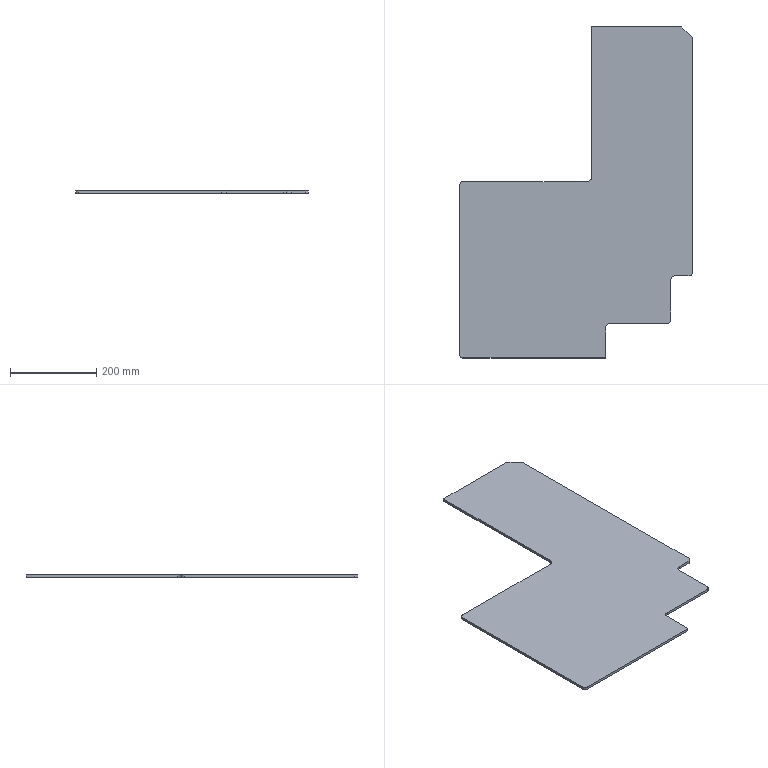Part | SolidWorks | features FlatPattern 1, SMBaseFlange 1, SheetMetal 1 | 1 solid | 24 faces | box 538 x 768 x 6 mm | volume 1689315 mm3 | plane 13 | cylinder 11 | commonest cylinder face diameters 15 x6 21 x3 3 x2
STEP:
#1=CARTESIAN_POINT('',(215.211,367.287,0.));
#2=VERTEX_POINT('',#1);
#3=CARTESIAN_POINT('',(209.908,369.483,0.));
#4=VERTEX_POINT('',#3);
#5=CARTESIAN_POINT('',(209.908,361.983,0.));
#6=DIRECTION('',(0.,0.,1.));
#7=DIRECTION('',(1.,0.,0.));
#8=AXIS2_PLACEMENT_3D('',#5,#6,#7);
#9=CIRCLE('',#8,7.5);
#10=EDGE_CURVE('',#2,#4,#9,.T.);
#11=ORIENTED_EDGE('',*,*,#10,.F.);
#12=CARTESIAN_POINT('',(215.211,367.287,-6.));
#13=VERTEX_POINT('',#12);
#14=CARTESIAN_POINT('',(215.211,367.287,-6.));
#15=DIRECTION('',(0.,0.,1.));
#16=VECTOR('',#15,1000.);
#17=LINE('',#14,#16);
#18=EDGE_CURVE('',#13,#2,#17,.T.);
#19=ORIENTED_EDGE('',*,*,#18,.F.);
#20=CARTESIAN_POINT('',(209.908,369.483,-6.));
#21=VERTEX_POINT('',#20);
#22=CARTESIAN_POINT('',(209.908,361.983,-6.));
#23=DIRECTION('',(0.,0.,1.));
#24=DIRECTION('',(1.,0.,0.));
#25=AXIS2_PLACEMENT_3D('',#22,#23,#24);
#26=CIRCLE('',#25,7.5);
#27=EDGE_CURVE('',#13,#21,#26,.T.);
#28=ORIENTED_EDGE('',*,*,#27,.T.);
#29=CARTESIAN_POINT('',(209.908,369.483,-6.));
#30=DIRECTION('',(0.,0.,1.));
#31=VECTOR('',#30,1000.);
#32=LINE('',#29,#31);
#33=EDGE_CURVE('',#21,#4,#32,.T.);
#34=ORIENTED_EDGE('',*,*,#33,.T.);
#35=EDGE_LOOP('',(#11,#19,#28,#34));
#36=FACE_OUTER_BOUND('',#35,.T.);
#37=CARTESIAN_POINT('',(209.908,361.983,-6.));
#38=DIRECTION('',(0.,0.,1.));
#39=DIRECTION('',(1.,0.,0.));
#40=AXIS2_PLACEMENT_3D('',#37,#38,#39);
#41=CYLINDRICAL_SURFACE('',#40,7.5);
#42=ADVANCED_FACE('',(#36),#41,.T.);
#43=CARTESIAN_POINT('',(237.303,345.195,0.));
#44=VERTEX_POINT('',#43);
#45=CARTESIAN_POINT('',(237.303,345.195,0.));
#46=DIRECTION('',(-0.7071,0.7071,0.));
#47=VECTOR('',#46,1000.);
#48=LINE('',#45,#47);
#49=EDGE_CURVE('',#44,#2,#48,.T.);
#50=ORIENTED_EDGE('',*,*,#49,.F.);
#51=CARTESIAN_POINT('',(237.303,345.195,-6.));
#52=VERTEX_POINT('',#51);
#53=CARTESIAN_POINT('',(237.303,345.195,-6.));
#54=DIRECTION('',(0.,0.,1.));
#55=VECTOR('',#54,1000.);
#56=LINE('',#53,#55);
#57=EDGE_CURVE('',#52,#44,#56,.T.);
#58=ORIENTED_EDGE('',*,*,#57,.F.);
#59=CARTESIAN_POINT('',(237.303,345.195,-6.));
#60=DIRECTION('',(-0.7071,0.7071,0.));
#61=VECTOR('',#60,1000.);
#62=LINE('',#59,#61);
#63=EDGE_CURVE('',#52,#13,#62,.T.);
#64=ORIENTED_EDGE('',*,*,#63,.T.);
#65=ORIENTED_EDGE('',*,*,#18,.T.);
#66=EDGE_LOOP('',(#50,#58,#64,#65));
#67=FACE_OUTER_BOUND('',#66,.T.);
#68=CARTESIAN_POINT('',(237.303,345.195,-6.));
#69=DIRECTION('',(0.7071,0.7071,0.));
#70=DIRECTION('',(-0.7071,0.7071,0.));
#71=AXIS2_PLACEMENT_3D('',#68,#69,#70);
#72=PLANE('',#71);
#73=ADVANCED_FACE('',(#67),#72,.T.);
#74=CARTESIAN_POINT('',(239.5,339.892,0.));
#75=VERTEX_POINT('',#74);
#76=CARTESIAN_POINT('',(232.,339.892,0.));
#77=DIRECTION('',(0.,0.,1.));
#78=DIRECTION('',(1.,0.,0.));
#79=AXIS2_PLACEMENT_3D('',#76,#77,#78);
#80=CIRCLE('',#79,7.5);
#81=EDGE_CURVE('',#75,#44,#80,.T.);
#82=ORIENTED_EDGE('',*,*,#81,.F.);
#83=CARTESIAN_POINT('',(239.5,339.892,-6.));
#84=VERTEX_POINT('',#83);
#85=CARTESIAN_POINT('',(239.5,339.892,-6.));
#86=DIRECTION('',(0.,0.,1.));
#87=VECTOR('',#86,1000.);
#88=LINE('',#85,#87);
#89=EDGE_CURVE('',#84,#75,#88,.T.);
#90=ORIENTED_EDGE('',*,*,#89,.F.);
#91=CARTESIAN_POINT('',(232.,339.892,-6.));
#92=DIRECTION('',(0.,0.,1.));
#93=DIRECTION('',(1.,0.,0.));
#94=AXIS2_PLACEMENT_3D('',#91,#92,#93);
#95=CIRCLE('',#94,7.5);
#96=EDGE_CURVE('',#84,#52,#95,.T.);
#97=ORIENTED_EDGE('',*,*,#96,.T.);
#98=ORIENTED_EDGE('',*,*,#57,.T.);
#99=EDGE_LOOP('',(#82,#90,#97,#98));
#100=FACE_OUTER_BOUND('',#99,.T.);
#101=CARTESIAN_POINT('',(232.,339.892,-6.));
#102=DIRECTION('',(0.,0.,1.));
#103=DIRECTION('',(1.,0.,0.));
#104=AXIS2_PLACEMENT_3D('',#101,#102,#103);
#105=CYLINDRICAL_SURFACE('',#104,7.5);
#106=ADVANCED_FACE('',(#100),#105,.T.);
#107=CARTESIAN_POINT('',(239.5,-201.017,0.));
#108=VERTEX_POINT('',#107);
#109=CARTESIAN_POINT('',(239.5,-201.017,0.));
#110=DIRECTION('',(0.,1.,0.));
#111=VECTOR('',#110,1000.);
#112=LINE('',#109,#111);
#113=EDGE_CURVE('',#108,#75,#112,.T.);
#114=ORIENTED_EDGE('',*,*,#113,.F.);
#115=CARTESIAN_POINT('',(239.5,-201.017,-6.));
#116=VERTEX_POINT('',#115);
#117=CARTESIAN_POINT('',(239.5,-201.017,-6.));
#118=DIRECTION('',(0.,0.,1.));
#119=VECTOR('',#118,1000.);
#120=LINE('',#117,#119);
#121=EDGE_CURVE('',#116,#108,#120,.T.);
#122=ORIENTED_EDGE('',*,*,#121,.F.);
#123=CARTESIAN_POINT('',(239.5,-201.017,-6.));
#124=DIRECTION('',(0.,1.,0.));
#125=VECTOR('',#124,1000.);
#126=LINE('',#123,#125);
#127=EDGE_CURVE('',#116,#84,#126,.T.);
#128=ORIENTED_EDGE('',*,*,#127,.T.);
#129=ORIENTED_EDGE('',*,*,#89,.T.);
#130=EDGE_LOOP('',(#114,#122,#128,#129));
#131=FACE_OUTER_BOUND('',#130,.T.);
#132=CARTESIAN_POINT('',(239.5,-201.017,-6.));
#133=DIRECTION('',(1.,0.,0.));
#134=DIRECTION('',(0.,0.,-1.));
#135=AXIS2_PLACEMENT_3D('',#132,#133,#134);
#136=PLANE('',#135);
#137=ADVANCED_FACE('',(#131),#136,.T.);
#138=CARTESIAN_POINT('',(232.,-208.517,0.));
#139=VERTEX_POINT('',#138);
#140=CARTESIAN_POINT('',(232.,-201.017,0.));
#141=DIRECTION('',(0.,0.,1.));
#142=DIRECTION('',(-1.,0.,0.));
#143=AXIS2_PLACEMENT_3D('',#140,#141,#142);
#144=CIRCLE('',#143,7.5);
#145=EDGE_CURVE('',#139,#108,#144,.T.);
#146=ORIENTED_EDGE('',*,*,#145,.F.);
#147=CARTESIAN_POINT('',(232.,-208.517,-6.));
#148=VERTEX_POINT('',#147);
#149=CARTESIAN_POINT('',(232.,-208.517,-6.));
#150=DIRECTION('',(0.,0.,1.));
#151=VECTOR('',#150,1000.);
#152=LINE('',#149,#151);
#153=EDGE_CURVE('',#148,#139,#152,.T.);
#154=ORIENTED_EDGE('',*,*,#153,.F.);
#155=CARTESIAN_POINT('',(232.,-201.017,-6.));
#156=DIRECTION('',(0.,0.,1.));
#157=DIRECTION('',(-1.,0.,0.));
#158=AXIS2_PLACEMENT_3D('',#155,#156,#157);
#159=CIRCLE('',#158,7.5);
#160=EDGE_CURVE('',#148,#116,#159,.T.);
#161=ORIENTED_EDGE('',*,*,#160,.T.);
#162=ORIENTED_EDGE('',*,*,#121,.T.);
#163=EDGE_LOOP('',(#146,#154,#161,#162));
#164=FACE_OUTER_BOUND('',#163,.T.);
#165=CARTESIAN_POINT('',(232.,-201.017,-6.));
#166=DIRECTION('',(0.,0.,1.));
#167=DIRECTION('',(1.,0.,0.));
#168=AXIS2_PLACEMENT_3D('',#165,#166,#167);
#169=CYLINDRICAL_SURFACE('',#168,7.5);
#170=ADVANCED_FACE('',(#164),#169,.T.);
#171=CARTESIAN_POINT('',(200.,-208.517,0.));
#172=VERTEX_POINT('',#171);
#173=CARTESIAN_POINT('',(200.,-208.517,0.));
#174=DIRECTION('',(1.,0.,0.));
#175=VECTOR('',#174,1000.);
#176=LINE('',#173,#175);
#177=EDGE_CURVE('',#172,#139,#176,.T.);
#178=ORIENTED_EDGE('',*,*,#177,.F.);
#179=CARTESIAN_POINT('',(200.,-208.517,-6.));
#180=VERTEX_POINT('',#179);
#181=CARTESIAN_POINT('',(200.,-208.517,-6.));
#182=DIRECTION('',(0.,0.,1.));
#183=VECTOR('',#182,1000.);
#184=LINE('',#181,#183);
#185=EDGE_CURVE('',#180,#172,#184,.T.);
#186=ORIENTED_EDGE('',*,*,#185,.F.);
#187=CARTESIAN_POINT('',(200.,-208.517,-6.));
#188=DIRECTION('',(1.,0.,0.));
#189=VECTOR('',#188,1000.);
#190=LINE('',#187,#189);
#191=EDGE_CURVE('',#180,#148,#190,.T.);
#192=ORIENTED_EDGE('',*,*,#191,.T.);
#193=ORIENTED_EDGE('',*,*,#153,.T.);
#194=EDGE_LOOP('',(#178,#186,#192,#193));
#195=FACE_OUTER_BOUND('',#194,.T.);
#196=CARTESIAN_POINT('',(200.,-208.517,-6.));
#197=DIRECTION('',(0.,-1.,0.));
#198=DIRECTION('',(0.,0.,-1.));
#199=AXIS2_PLACEMENT_3D('',#196,#197,#198);
#200=PLANE('',#199);
#201=ADVANCED_FACE('',(#195),#200,.T.);
#202=CARTESIAN_POINT('',(189.5,-219.017,0.));
#203=VERTEX_POINT('',#202);
#204=CARTESIAN_POINT('',(200.,-219.017,0.));
#205=DIRECTION('',(0.,0.,-1.));
#206=DIRECTION('',(1.,0.,0.));
#207=AXIS2_PLACEMENT_3D('',#204,#205,#206);
#208=CIRCLE('',#207,10.5);
#209=EDGE_CURVE('',#203,#172,#208,.T.);
#210=ORIENTED_EDGE('',*,*,#209,.F.);
#211=CARTESIAN_POINT('',(189.5,-219.017,-6.));
#212=VERTEX_POINT('',#211);
#213=CARTESIAN_POINT('',(189.5,-219.017,-6.));
#214=DIRECTION('',(0.,0.,1.));
#215=VECTOR('',#214,1000.);
#216=LINE('',#213,#215);
#217=EDGE_CURVE('',#212,#203,#216,.T.);
#218=ORIENTED_EDGE('',*,*,#217,.F.);
#219=CARTESIAN_POINT('',(200.,-219.017,-6.));
#220=DIRECTION('',(0.,0.,-1.));
#221=DIRECTION('',(1.,0.,0.));
#222=AXIS2_PLACEMENT_3D('',#219,#220,#221);
#223=CIRCLE('',#222,10.5);
#224=EDGE_CURVE('',#212,#180,#223,.T.);
#225=ORIENTED_EDGE('',*,*,#224,.T.);
#226=ORIENTED_EDGE('',*,*,#185,.T.);
#227=EDGE_LOOP('',(#210,#218,#225,#226));
#228=FACE_OUTER_BOUND('',#227,.T.);
#229=CARTESIAN_POINT('',(200.,-219.017,-6.));
#230=DIRECTION('',(0.,0.,1.));
#231=DIRECTION('',(1.,0.,0.));
#232=AXIS2_PLACEMENT_3D('',#229,#230,#231);
#233=CYLINDRICAL_SURFACE('',#232,10.5);
#234=ADVANCED_FACE('',(#228),#233,.F.);
#235=CARTESIAN_POINT('',(189.5,-311.017,0.));
#236=VERTEX_POINT('',#235);
#237=CARTESIAN_POINT('',(189.5,-311.017,0.));
#238=DIRECTION('',(0.,1.,0.));
#239=VECTOR('',#238,1000.);
#240=LINE('',#237,#239);
#241=EDGE_CURVE('',#236,#203,#240,.T.);
#242=ORIENTED_EDGE('',*,*,#241,.F.);
#243=CARTESIAN_POINT('',(189.5,-311.017,-6.));
#244=VERTEX_POINT('',#243);
#245=CARTESIAN_POINT('',(189.5,-311.017,-6.));
#246=DIRECTION('',(0.,0.,1.));
#247=VECTOR('',#246,1000.);
#248=LINE('',#245,#247);
#249=EDGE_CURVE('',#244,#236,#248,.T.);
#250=ORIENTED_EDGE('',*,*,#249,.F.);
#251=CARTESIAN_POINT('',(189.5,-311.017,-6.));
#252=DIRECTION('',(0.,1.,0.));
#253=VECTOR('',#252,1000.);
#254=LINE('',#251,#253);
#255=EDGE_CURVE('',#244,#212,#254,.T.);
#256=ORIENTED_EDGE('',*,*,#255,.T.);
#257=ORIENTED_EDGE('',*,*,#217,.T.);
#258=EDGE_LOOP('',(#242,#250,#256,#257));
#259=FACE_OUTER_BOUND('',#258,.T.);
#260=CARTESIAN_POINT('',(189.5,-311.017,-6.));
#261=DIRECTION('',(1.,0.,0.));
#262=DIRECTION('',(0.,0.,-1.));
#263=AXIS2_PLACEMENT_3D('',#260,#261,#262);
#264=PLANE('',#263);
#265=ADVANCED_FACE('',(#259),#264,.T.);
#266=CARTESIAN_POINT('',(182.,-318.517,0.));
#267=VERTEX_POINT('',#266);
#268=CARTESIAN_POINT('',(182.,-311.017,0.));
#269=DIRECTION('',(0.,0.,1.));
#270=DIRECTION('',(-1.,0.,0.));
#271=AXIS2_PLACEMENT_3D('',#268,#269,#270);
#272=CIRCLE('',#271,7.5);
#273=EDGE_CURVE('',#267,#236,#272,.T.);
#274=ORIENTED_EDGE('',*,*,#273,.F.);
#275=CARTESIAN_POINT('',(182.,-318.517,-6.));
#276=VERTEX_POINT('',#275);
#277=CARTESIAN_POINT('',(182.,-318.517,-6.));
#278=DIRECTION('',(0.,0.,1.));
#279=VECTOR('',#278,1000.);
#280=LINE('',#277,#279);
#281=EDGE_CURVE('',#276,#267,#280,.T.);
#282=ORIENTED_EDGE('',*,*,#281,.F.);
#283=CARTESIAN_POINT('',(182.,-311.017,-6.));
#284=DIRECTION('',(0.,0.,1.));
#285=DIRECTION('',(-1.,0.,0.));
#286=AXIS2_PLACEMENT_3D('',#283,#284,#285);
#287=CIRCLE('',#286,7.5);
#288=EDGE_CURVE('',#276,#244,#287,.T.);
#289=ORIENTED_EDGE('',*,*,#288,.T.);
#290=ORIENTED_EDGE('',*,*,#249,.T.);
#291=EDGE_LOOP('',(#274,#282,#289,#290));
#292=FACE_OUTER_BOUND('',#291,.T.);
#293=CARTESIAN_POINT('',(182.,-311.017,-6.));
#294=DIRECTION('',(0.,0.,1.));
#295=DIRECTION('',(1.,0.,0.));
#296=AXIS2_PLACEMENT_3D('',#293,#294,#295);
#297=CYLINDRICAL_SURFACE('',#296,7.5);
#298=ADVANCED_FACE('',(#292),#297,.T.);
#299=CARTESIAN_POINT('',(50.,-318.517,0.));
#300=VERTEX_POINT('',#299);
#301=CARTESIAN_POINT('',(50.,-318.517,0.));
#302=DIRECTION('',(1.,0.,0.));
#303=VECTOR('',#302,1000.);
#304=LINE('',#301,#303);
#305=EDGE_CURVE('',#300,#267,#304,.T.);
#306=ORIENTED_EDGE('',*,*,#305,.F.);
#307=CARTESIAN_POINT('',(50.,-318.517,-6.));
#308=VERTEX_POINT('',#307);
#309=CARTESIAN_POINT('',(50.,-318.517,-6.));
#310=DIRECTION('',(0.,0.,1.));
#311=VECTOR('',#310,1000.);
#312=LINE('',#309,#311);
#313=EDGE_CURVE('',#308,#300,#312,.T.);
#314=ORIENTED_EDGE('',*,*,#313,.F.);
#315=CARTESIAN_POINT('',(50.,-318.517,-6.));
#316=DIRECTION('',(1.,0.,0.));
#317=VECTOR('',#316,1000.);
#318=LINE('',#315,#317);
#319=EDGE_CURVE('',#308,#276,#318,.T.);
#320=ORIENTED_EDGE('',*,*,#319,.T.);
#321=ORIENTED_EDGE('',*,*,#281,.T.);
#322=EDGE_LOOP('',(#306,#314,#320,#321));
#323=FACE_OUTER_BOUND('',#322,.T.);
#324=CARTESIAN_POINT('',(50.,-318.517,-6.));
#325=DIRECTION('',(0.,-1.,0.));
#326=DIRECTION('',(1.,0.,0.));
#327=AXIS2_PLACEMENT_3D('',#324,#325,#326);
#328=PLANE('',#327);
#329=ADVANCED_FACE('',(#323),#328,.T.);
#330=CARTESIAN_POINT('',(39.5,-329.017,0.));
#331=VERTEX_POINT('',#330);
#332=CARTESIAN_POINT('',(50.,-329.017,0.));
#333=DIRECTION('',(0.,0.,-1.));
#334=DIRECTION('',(1.,0.,0.));
#335=AXIS2_PLACEMENT_3D('',#332,#333,#334);
#336=CIRCLE('',#335,10.5);
#337=EDGE_CURVE('',#331,#300,#336,.T.);
#338=ORIENTED_EDGE('',*,*,#337,.F.);
#339=CARTESIAN_POINT('',(39.5,-329.017,-6.));
#340=VERTEX_POINT('',#339);
#341=CARTESIAN_POINT('',(39.5,-329.017,-6.));
#342=DIRECTION('',(0.,0.,1.));
#343=VECTOR('',#342,1000.);
#344=LINE('',#341,#343);
#345=EDGE_CURVE('',#340,#331,#344,.T.);
#346=ORIENTED_EDGE('',*,*,#345,.F.);
#347=CARTESIAN_POINT('',(50.,-329.017,-6.));
#348=DIRECTION('',(0.,0.,-1.));
#349=DIRECTION('',(1.,0.,0.));
#350=AXIS2_PLACEMENT_3D('',#347,#348,#349);
#351=CIRCLE('',#350,10.5);
#352=EDGE_CURVE('',#340,#308,#351,.T.);
#353=ORIENTED_EDGE('',*,*,#352,.T.);
#354=ORIENTED_EDGE('',*,*,#313,.T.);
#355=EDGE_LOOP('',(#338,#346,#353,#354));
#356=FACE_OUTER_BOUND('',#355,.T.);
#357=CARTESIAN_POINT('',(50.,-329.017,-6.));
#358=DIRECTION('',(0.,0.,1.));
#359=DIRECTION('',(1.,0.,0.));
#360=AXIS2_PLACEMENT_3D('',#357,#358,#359);
#361=CYLINDRICAL_SURFACE('',#360,10.5);
#362=ADVANCED_FACE('',(#356),#361,.F.);
#363=CARTESIAN_POINT('',(39.5,-397.017,0.));
#364=VERTEX_POINT('',#363);
#365=CARTESIAN_POINT('',(39.5,-397.017,0.));
#366=DIRECTION('',(0.,1.,0.));
#367=VECTOR('',#366,1000.);
#368=LINE('',#365,#367);
#369=EDGE_CURVE('',#364,#331,#368,.T.);
#370=ORIENTED_EDGE('',*,*,#369,.F.);
#371=CARTESIAN_POINT('',(39.5,-397.017,-6.));
#372=VERTEX_POINT('',#371);
#373=CARTESIAN_POINT('',(39.5,-397.017,-6.));
#374=DIRECTION('',(0.,0.,1.));
#375=VECTOR('',#374,1000.);
#376=LINE('',#373,#375);
#377=EDGE_CURVE('',#372,#364,#376,.T.);
#378=ORIENTED_EDGE('',*,*,#377,.F.);
#379=CARTESIAN_POINT('',(39.5,-397.017,-6.));
#380=DIRECTION('',(0.,1.,0.));
#381=VECTOR('',#380,1000.);
#382=LINE('',#379,#381);
#383=EDGE_CURVE('',#372,#340,#382,.T.);
#384=ORIENTED_EDGE('',*,*,#383,.T.);
#385=ORIENTED_EDGE('',*,*,#345,.T.);
#386=EDGE_LOOP('',(#370,#378,#384,#385));
#387=FACE_OUTER_BOUND('',#386,.T.);
#388=CARTESIAN_POINT('',(39.5,-397.017,-6.));
#389=DIRECTION('',(1.,0.,0.));
#390=DIRECTION('',(0.,0.,-1.));
#391=AXIS2_PLACEMENT_3D('',#388,#389,#390);
#392=PLANE('',#391);
#393=ADVANCED_FACE('',(#387),#392,.T.);
#394=CARTESIAN_POINT('',(38.,-398.517,0.));
#395=VERTEX_POINT('',#394);
#396=CARTESIAN_POINT('',(38.,-397.017,0.));
#397=DIRECTION('',(0.,0.,1.));
#398=DIRECTION('',(-1.,0.,0.));
#399=AXIS2_PLACEMENT_3D('',#396,#397,#398);
#400=CIRCLE('',#399,1.5);
#401=EDGE_CURVE('',#395,#364,#400,.T.);
#402=ORIENTED_EDGE('',*,*,#401,.F.);
#403=CARTESIAN_POINT('',(38.,-398.517,-6.));
#404=VERTEX_POINT('',#403);
#405=CARTESIAN_POINT('',(38.,-398.517,-6.));
#406=DIRECTION('',(0.,0.,1.));
#407=VECTOR('',#406,1000.);
#408=LINE('',#405,#407);
#409=EDGE_CURVE('',#404,#395,#408,.T.);
#410=ORIENTED_EDGE('',*,*,#409,.F.);
#411=CARTESIAN_POINT('',(38.,-397.017,-6.));
#412=DIRECTION('',(0.,0.,1.));
#413=DIRECTION('',(-1.,0.,0.));
#414=AXIS2_PLACEMENT_3D('',#411,#412,#413);
#415=CIRCLE('',#414,1.5);
#416=EDGE_CURVE('',#404,#372,#415,.T.);
#417=ORIENTED_EDGE('',*,*,#416,.T.);
#418=ORIENTED_EDGE('',*,*,#377,.T.);
#419=EDGE_LOOP('',(#402,#410,#417,#418));
#420=FACE_OUTER_BOUND('',#419,.T.);
#421=CARTESIAN_POINT('',(38.,-397.017,-6.));
#422=DIRECTION('',(0.,0.,1.));
#423=DIRECTION('',(1.,0.,0.));
#424=AXIS2_PLACEMENT_3D('',#421,#422,#423);
#425=CYLINDRICAL_SURFACE('',#424,1.5);
#426=ADVANCED_FACE('',(#420),#425,.T.);
#427=CARTESIAN_POINT('',(-291.,-398.517,0.));
#428=VERTEX_POINT('',#427);
#429=CARTESIAN_POINT('',(38.,-398.517,0.));
#430=DIRECTION('',(1.,0.,0.));
#431=VECTOR('',#430,1000.);
#432=LINE('',#429,#431);
#433=EDGE_CURVE('',#428,#395,#432,.T.);
#434=ORIENTED_EDGE('',*,*,#433,.F.);
#435=CARTESIAN_POINT('',(-291.,-398.517,-6.));
#436=VERTEX_POINT('',#435);
#437=CARTESIAN_POINT('',(-291.,-398.517,-6.));
#438=DIRECTION('',(0.,0.,1.));
#439=VECTOR('',#438,1000.);
#440=LINE('',#437,#439);
#441=EDGE_CURVE('',#436,#428,#440,.T.);
#442=ORIENTED_EDGE('',*,*,#441,.F.);
#443=CARTESIAN_POINT('',(38.,-398.517,-6.));
#444=DIRECTION('',(1.,0.,0.));
#445=VECTOR('',#444,1000.);
#446=LINE('',#443,#445);
#447=EDGE_CURVE('',#436,#404,#446,.T.);
#448=ORIENTED_EDGE('',*,*,#447,.T.);
#449=ORIENTED_EDGE('',*,*,#409,.T.);
#450=EDGE_LOOP('',(#434,#442,#448,#449));
#451=FACE_OUTER_BOUND('',#450,.T.);
#452=CARTESIAN_POINT('',(38.,-398.517,-6.));
#453=DIRECTION('',(0.,-1.,0.));
#454=DIRECTION('',(1.,0.,0.));
#455=AXIS2_PLACEMENT_3D('',#452,#453,#454);
#456=PLANE('',#455);
#457=ADVANCED_FACE('',(#451),#456,.T.);
#458=CARTESIAN_POINT('',(-298.5,-391.017,0.));
#459=VERTEX_POINT('',#458);
#460=CARTESIAN_POINT('',(-291.,-391.017,0.));
#461=DIRECTION('',(0.,0.,1.));
#462=DIRECTION('',(-1.,0.,0.));
#463=AXIS2_PLACEMENT_3D('',#460,#461,#462);
#464=CIRCLE('',#463,7.5);
#465=EDGE_CURVE('',#459,#428,#464,.T.);
#466=ORIENTED_EDGE('',*,*,#465,.F.);
#467=CARTESIAN_POINT('',(-298.5,-391.017,-6.));
#468=VERTEX_POINT('',#467);
#469=CARTESIAN_POINT('',(-298.5,-391.017,-6.));
#470=DIRECTION('',(0.,0.,1.));
#471=VECTOR('',#470,1000.);
#472=LINE('',#469,#471);
#473=EDGE_CURVE('',#468,#459,#472,.T.);
#474=ORIENTED_EDGE('',*,*,#473,.F.);
#475=CARTESIAN_POINT('',(-291.,-391.017,-6.));
#476=DIRECTION('',(0.,0.,1.));
#477=DIRECTION('',(-1.,0.,0.));
#478=AXIS2_PLACEMENT_3D('',#475,#476,#477);
#479=CIRCLE('',#478,7.5);
#480=EDGE_CURVE('',#468,#436,#479,.T.);
#481=ORIENTED_EDGE('',*,*,#480,.T.);
#482=ORIENTED_EDGE('',*,*,#441,.T.);
#483=EDGE_LOOP('',(#466,#474,#481,#482));
#484=FACE_OUTER_BOUND('',#483,.T.);
#485=CARTESIAN_POINT('',(-291.,-391.017,-6.));
#486=DIRECTION('',(0.,0.,1.));
#487=DIRECTION('',(1.,0.,0.));
#488=AXIS2_PLACEMENT_3D('',#485,#486,#487);
#489=CYLINDRICAL_SURFACE('',#488,7.5);
#490=ADVANCED_FACE('',(#484),#489,.T.);
#491=CARTESIAN_POINT('',(-298.5,1.983,0.));
#492=VERTEX_POINT('',#491);
#493=CARTESIAN_POINT('',(-298.5,-391.017,0.));
#494=DIRECTION('',(0.,-1.,0.));
#495=VECTOR('',#494,1000.);
#496=LINE('',#493,#495);
#497=EDGE_CURVE('',#492,#459,#496,.T.);
#498=ORIENTED_EDGE('',*,*,#497,.F.);
#499=CARTESIAN_POINT('',(-298.5,1.983,-6.));
#500=VERTEX_POINT('',#499);
#501=CARTESIAN_POINT('',(-298.5,1.983,-6.));
#502=DIRECTION('',(0.,0.,1.));
#503=VECTOR('',#502,1000.);
#504=LINE('',#501,#503);
#505=EDGE_CURVE('',#500,#492,#504,.T.);
#506=ORIENTED_EDGE('',*,*,#505,.F.);
#507=CARTESIAN_POINT('',(-298.5,-391.017,-6.));
#508=DIRECTION('',(0.,-1.,0.));
#509=VECTOR('',#508,1000.);
#510=LINE('',#507,#509);
#511=EDGE_CURVE('',#500,#468,#510,.T.);
#512=ORIENTED_EDGE('',*,*,#511,.T.);
#513=ORIENTED_EDGE('',*,*,#473,.T.);
#514=EDGE_LOOP('',(#498,#506,#512,#513));
#515=FACE_OUTER_BOUND('',#514,.T.);
#516=CARTESIAN_POINT('',(-298.5,-391.017,-6.));
#517=DIRECTION('',(-1.,0.,0.));
#518=DIRECTION('',(0.,-1.,0.));
#519=AXIS2_PLACEMENT_3D('',#516,#517,#518);
#520=PLANE('',#519);
#521=ADVANCED_FACE('',(#515),#520,.T.);
#522=CARTESIAN_POINT('',(-291.,9.483,0.));
#523=VERTEX_POINT('',#522);
#524=CARTESIAN_POINT('',(-291.,1.983,0.));
#525=DIRECTION('',(0.,0.,1.));
#526=DIRECTION('',(-1.,0.,0.));
#527=AXIS2_PLACEMENT_3D('',#524,#525,#526);
#528=CIRCLE('',#527,7.5);
#529=EDGE_CURVE('',#523,#492,#528,.T.);
#530=ORIENTED_EDGE('',*,*,#529,.F.);
#531=CARTESIAN_POINT('',(-291.,9.483,-6.));
#532=VERTEX_POINT('',#531);
#533=CARTESIAN_POINT('',(-291.,9.483,-6.));
#534=DIRECTION('',(0.,0.,1.));
#535=VECTOR('',#534,1000.);
#536=LINE('',#533,#535);
#537=EDGE_CURVE('',#532,#523,#536,.T.);
#538=ORIENTED_EDGE('',*,*,#537,.F.);
#539=CARTESIAN_POINT('',(-291.,1.983,-6.));
#540=DIRECTION('',(0.,0.,1.));
#541=DIRECTION('',(-1.,0.,0.));
#542=AXIS2_PLACEMENT_3D('',#539,#540,#541);
#543=CIRCLE('',#542,7.5);
#544=EDGE_CURVE('',#532,#500,#543,.T.);
#545=ORIENTED_EDGE('',*,*,#544,.T.);
#546=ORIENTED_EDGE('',*,*,#505,.T.);
#547=EDGE_LOOP('',(#530,#538,#545,#546));
#548=FACE_OUTER_BOUND('',#547,.T.);
#549=CARTESIAN_POINT('',(-291.,1.983,-6.));
#550=DIRECTION('',(0.,0.,1.));
#551=DIRECTION('',(1.,0.,0.));
#552=AXIS2_PLACEMENT_3D('',#549,#550,#551);
#553=CYLINDRICAL_SURFACE('',#552,7.5);
#554=ADVANCED_FACE('',(#548),#553,.T.);
#555=CARTESIAN_POINT('',(-4.,9.483,0.));
#556=VERTEX_POINT('',#555);
#557=CARTESIAN_POINT('',(-291.,9.483,0.));
#558=DIRECTION('',(-1.,0.,0.));
#559=VECTOR('',#558,1000.);
#560=LINE('',#557,#559);
#561=EDGE_CURVE('',#556,#523,#560,.T.);
#562=ORIENTED_EDGE('',*,*,#561,.F.);
#563=CARTESIAN_POINT('',(-4.,9.483,-6.));
#564=VERTEX_POINT('',#563);
#565=CARTESIAN_POINT('',(-4.,9.483,-6.));
#566=DIRECTION('',(0.,0.,1.));
#567=VECTOR('',#566,1000.);
#568=LINE('',#565,#567);
#569=EDGE_CURVE('',#564,#556,#568,.T.);
#570=ORIENTED_EDGE('',*,*,#569,.F.);
#571=CARTESIAN_POINT('',(-291.,9.483,-6.));
#572=DIRECTION('',(-1.,0.,0.));
#573=VECTOR('',#572,1000.);
#574=LINE('',#571,#573);
#575=EDGE_CURVE('',#564,#532,#574,.T.);
#576=ORIENTED_EDGE('',*,*,#575,.T.);
#577=ORIENTED_EDGE('',*,*,#537,.T.);
#578=EDGE_LOOP('',(#562,#570,#576,#577));
#579=FACE_OUTER_BOUND('',#578,.T.);
#580=CARTESIAN_POINT('',(-291.,9.483,-6.));
#581=DIRECTION('',(0.,1.,0.));
#582=DIRECTION('',(0.,0.,1.));
#583=AXIS2_PLACEMENT_3D('',#580,#581,#582);
#584=PLANE('',#583);
#585=ADVANCED_FACE('',(#579),#584,.T.);
#586=CARTESIAN_POINT('',(6.5,19.983,0.));
#587=VERTEX_POINT('',#586);
#588=CARTESIAN_POINT('',(-4.,19.983,0.));
#589=DIRECTION('',(0.,0.,-1.));
#590=DIRECTION('',(-1.,0.,0.));
#591=AXIS2_PLACEMENT_3D('',#588,#589,#590);
#592=CIRCLE('',#591,10.5);
#593=EDGE_CURVE('',#587,#556,#592,.T.);
#594=ORIENTED_EDGE('',*,*,#593,.F.);
#595=CARTESIAN_POINT('',(6.5,19.983,-6.));
#596=VERTEX_POINT('',#595);
#597=CARTESIAN_POINT('',(6.5,19.983,-6.));
#598=DIRECTION('',(0.,0.,1.));
#599=VECTOR('',#598,1000.);
#600=LINE('',#597,#599);
#601=EDGE_CURVE('',#596,#587,#600,.T.);
#602=ORIENTED_EDGE('',*,*,#601,.F.);
#603=CARTESIAN_POINT('',(-4.,19.983,-6.));
#604=DIRECTION('',(0.,0.,-1.));
#605=DIRECTION('',(-1.,0.,0.));
#606=AXIS2_PLACEMENT_3D('',#603,#604,#605);
#607=CIRCLE('',#606,10.5);
#608=EDGE_CURVE('',#596,#564,#607,.T.);
#609=ORIENTED_EDGE('',*,*,#608,.T.);
#610=ORIENTED_EDGE('',*,*,#569,.T.);
#611=EDGE_LOOP('',(#594,#602,#609,#610));
#612=FACE_OUTER_BOUND('',#611,.T.);
#613=CARTESIAN_POINT('',(-4.,19.983,-6.));
#614=DIRECTION('',(0.,0.,1.));
#615=DIRECTION('',(1.,0.,0.));
#616=AXIS2_PLACEMENT_3D('',#613,#614,#615);
#617=CYLINDRICAL_SURFACE('',#616,10.5);
#618=ADVANCED_FACE('',(#612),#617,.F.);
#619=CARTESIAN_POINT('',(6.5,367.983,0.));
#620=VERTEX_POINT('',#619);
#621=CARTESIAN_POINT('',(6.5,19.983,0.));
#622=DIRECTION('',(0.,-1.,0.));
#623=VECTOR('',#622,1000.);
#624=LINE('',#621,#623);
#625=EDGE_CURVE('',#620,#587,#624,.T.);
#626=ORIENTED_EDGE('',*,*,#625,.F.);
#627=CARTESIAN_POINT('',(6.5,367.983,-6.));
#628=VERTEX_POINT('',#627);
#629=CARTESIAN_POINT('',(6.5,367.983,-6.));
#630=DIRECTION('',(0.,0.,1.));
#631=VECTOR('',#630,1000.);
#632=LINE('',#629,#631);
#633=EDGE_CURVE('',#628,#620,#632,.T.);
#634=ORIENTED_EDGE('',*,*,#633,.F.);
#635=CARTESIAN_POINT('',(6.5,19.983,-6.));
#636=DIRECTION('',(0.,-1.,0.));
#637=VECTOR('',#636,1000.);
#638=LINE('',#635,#637);
#639=EDGE_CURVE('',#628,#596,#638,.T.);
#640=ORIENTED_EDGE('',*,*,#639,.T.);
#641=ORIENTED_EDGE('',*,*,#601,.T.);
#642=EDGE_LOOP('',(#626,#634,#640,#641));
#643=FACE_OUTER_BOUND('',#642,.T.);
#644=CARTESIAN_POINT('',(6.5,19.983,-6.));
#645=DIRECTION('',(-1.,0.,0.));
#646=DIRECTION('',(0.,0.,1.));
#647=AXIS2_PLACEMENT_3D('',#644,#645,#646);
#648=PLANE('',#647);
#649=ADVANCED_FACE('',(#643),#648,.T.);
#650=CARTESIAN_POINT('',(8.,369.483,0.));
#651=VERTEX_POINT('',#650);
#652=CARTESIAN_POINT('',(8.,367.983,0.));
#653=DIRECTION('',(0.,0.,1.));
#654=DIRECTION('',(1.,0.,0.));
#655=AXIS2_PLACEMENT_3D('',#652,#653,#654);
#656=CIRCLE('',#655,1.5);
#657=EDGE_CURVE('',#651,#620,#656,.T.);
#658=ORIENTED_EDGE('',*,*,#657,.F.);
#659=CARTESIAN_POINT('',(8.,369.483,-6.));
#660=VERTEX_POINT('',#659);
#661=CARTESIAN_POINT('',(8.,369.483,-6.));
#662=DIRECTION('',(0.,0.,1.));
#663=VECTOR('',#662,1000.);
#664=LINE('',#661,#663);
#665=EDGE_CURVE('',#660,#651,#664,.T.);
#666=ORIENTED_EDGE('',*,*,#665,.F.);
#667=CARTESIAN_POINT('',(8.,367.983,-6.));
#668=DIRECTION('',(0.,0.,1.));
#669=DIRECTION('',(1.,0.,0.));
#670=AXIS2_PLACEMENT_3D('',#667,#668,#669);
#671=CIRCLE('',#670,1.5);
#672=EDGE_CURVE('',#660,#628,#671,.T.);
#673=ORIENTED_EDGE('',*,*,#672,.T.);
#674=ORIENTED_EDGE('',*,*,#633,.T.);
#675=EDGE_LOOP('',(#658,#666,#673,#674));
#676=FACE_OUTER_BOUND('',#675,.T.);
#677=CARTESIAN_POINT('',(8.,367.983,-6.));
#678=DIRECTION('',(0.,0.,1.));
#679=DIRECTION('',(1.,0.,0.));
#680=AXIS2_PLACEMENT_3D('',#677,#678,#679);
#681=CYLINDRICAL_SURFACE('',#680,1.5);
#682=ADVANCED_FACE('',(#676),#681,.T.);
#683=CARTESIAN_POINT('',(209.908,369.483,0.));
#684=DIRECTION('',(-1.,0.,0.));
#685=VECTOR('',#684,1000.);
#686=LINE('',#683,#685);
#687=EDGE_CURVE('',#4,#651,#686,.T.);
#688=ORIENTED_EDGE('',*,*,#687,.F.);
#689=ORIENTED_EDGE('',*,*,#33,.F.);
#690=CARTESIAN_POINT('',(209.908,369.483,-6.));
#691=DIRECTION('',(-1.,0.,0.));
#692=VECTOR('',#691,1000.);
#693=LINE('',#690,#692);
#694=EDGE_CURVE('',#21,#660,#693,.T.);
#695=ORIENTED_EDGE('',*,*,#694,.T.);
#696=ORIENTED_EDGE('',*,*,#665,.T.);
#697=EDGE_LOOP('',(#688,#689,#695,#696));
#698=FACE_OUTER_BOUND('',#697,.T.);
#699=CARTESIAN_POINT('',(209.908,369.483,-6.));
#700=DIRECTION('',(0.,1.,0.));
#701=DIRECTION('',(-1.,0.,0.));
#702=AXIS2_PLACEMENT_3D('',#699,#700,#701);
#703=PLANE('',#702);
#704=ADVANCED_FACE('',(#698),#703,.T.);
#705=ORIENTED_EDGE('',*,*,#27,.F.);
#706=ORIENTED_EDGE('',*,*,#63,.F.);
#707=ORIENTED_EDGE('',*,*,#96,.F.);
#708=ORIENTED_EDGE('',*,*,#127,.F.);
#709=ORIENTED_EDGE('',*,*,#160,.F.);
#710=ORIENTED_EDGE('',*,*,#191,.F.);
#711=ORIENTED_EDGE('',*,*,#224,.F.);
#712=ORIENTED_EDGE('',*,*,#255,.F.);
#713=ORIENTED_EDGE('',*,*,#288,.F.);
#714=ORIENTED_EDGE('',*,*,#319,.F.);
#715=ORIENTED_EDGE('',*,*,#352,.F.);
#716=ORIENTED_EDGE('',*,*,#383,.F.);
#717=ORIENTED_EDGE('',*,*,#416,.F.);
#718=ORIENTED_EDGE('',*,*,#447,.F.);
#719=ORIENTED_EDGE('',*,*,#480,.F.);
#720=ORIENTED_EDGE('',*,*,#511,.F.);
#721=ORIENTED_EDGE('',*,*,#544,.F.);
#722=ORIENTED_EDGE('',*,*,#575,.F.);
#723=ORIENTED_EDGE('',*,*,#608,.F.);
#724=ORIENTED_EDGE('',*,*,#639,.F.);
#725=ORIENTED_EDGE('',*,*,#672,.F.);
#726=ORIENTED_EDGE('',*,*,#694,.F.);
#727=EDGE_LOOP('',(#705,#706,#707,#708,#709,#710,#711,#712,#713,#714,#715,#716,#717,#718,#719,#720,#721,#722,#723,#724,#725,#726));
#728=FACE_OUTER_BOUND('',#727,.T.);
#729=CARTESIAN_POINT('',(209.908,361.983,-6.));
#730=DIRECTION('',(0.,0.,1.));
#731=DIRECTION('',(1.,0.,0.));
#732=AXIS2_PLACEMENT_3D('',#729,#730,#731);
#733=PLANE('',#732);
#734=ADVANCED_FACE('',(#728),#733,.F.);
#735=ORIENTED_EDGE('',*,*,#10,.T.);
#736=ORIENTED_EDGE('',*,*,#687,.T.);
#737=ORIENTED_EDGE('',*,*,#657,.T.);
#738=ORIENTED_EDGE('',*,*,#625,.T.);
#739=ORIENTED_EDGE('',*,*,#593,.T.);
#740=ORIENTED_EDGE('',*,*,#561,.T.);
#741=ORIENTED_EDGE('',*,*,#529,.T.);
#742=ORIENTED_EDGE('',*,*,#497,.T.);
#743=ORIENTED_EDGE('',*,*,#465,.T.);
#744=ORIENTED_EDGE('',*,*,#433,.T.);
#745=ORIENTED_EDGE('',*,*,#401,.T.);
#746=ORIENTED_EDGE('',*,*,#369,.T.);
#747=ORIENTED_EDGE('',*,*,#337,.T.);
#748=ORIENTED_EDGE('',*,*,#305,.T.);
#749=ORIENTED_EDGE('',*,*,#273,.T.);
#750=ORIENTED_EDGE('',*,*,#241,.T.);
#751=ORIENTED_EDGE('',*,*,#209,.T.);
#752=ORIENTED_EDGE('',*,*,#177,.T.);
#753=ORIENTED_EDGE('',*,*,#145,.T.);
#754=ORIENTED_EDGE('',*,*,#113,.T.);
#755=ORIENTED_EDGE('',*,*,#81,.T.);
#756=ORIENTED_EDGE('',*,*,#49,.T.);
#757=EDGE_LOOP('',(#735,#736,#737,#738,#739,#740,#741,#742,#743,#744,#745,#746,#747,#748,#749,#750,#751,#752,#753,#754,#755,#756));
#758=FACE_OUTER_BOUND('',#757,.T.);
#759=CARTESIAN_POINT('',(209.908,361.983,0.));
#760=DIRECTION('',(0.,0.,1.));
#761=DIRECTION('',(1.,0.,0.));
#762=AXIS2_PLACEMENT_3D('',#759,#760,#761);
#763=PLANE('',#762);
#764=ADVANCED_FACE('',(#758),#763,.T.);
#765=CLOSED_SHELL('',(#42,#73,#106,#137,#170,#201,#234,#265,#298,#329,#362,#393,#426,#457,#490,#521,#554,#585,#618,#649,#682,#704,#734,#764));
#766=MANIFOLD_SOLID_BREP('',#765);
#767=CARTESIAN_POINT('',(0.,0.,0.));
#768=DIRECTION('',(0.,0.,1.));
#769=DIRECTION('',(1.,0.,0.));
#770=AXIS2_PLACEMENT_3D('',#767,#768,#769);
#771=(LENGTH_UNIT()NAMED_UNIT(*)SI_UNIT(.MILLI.,.METRE.));
#772=UNCERTAINTY_MEASURE_WITH_UNIT(LENGTH_MEASURE(0.00001),#771,'','');
#773=(NAMED_UNIT(*)PLANE_ANGLE_UNIT()SI_UNIT($,.RADIAN.));
#774=(NAMED_UNIT(*)SI_UNIT($,.STERADIAN.)SOLID_ANGLE_UNIT());
#775=(GEOMETRIC_REPRESENTATION_CONTEXT(3)GLOBAL_UNCERTAINTY_ASSIGNED_CONTEXT((#772))GLOBAL_UNIT_ASSIGNED_CONTEXT((#771,#773,#774))REPRESENTATION_CONTEXT('',''));
#776=ADVANCED_BREP_SHAPE_REPRESENTATION('',(#766,#770),#775);